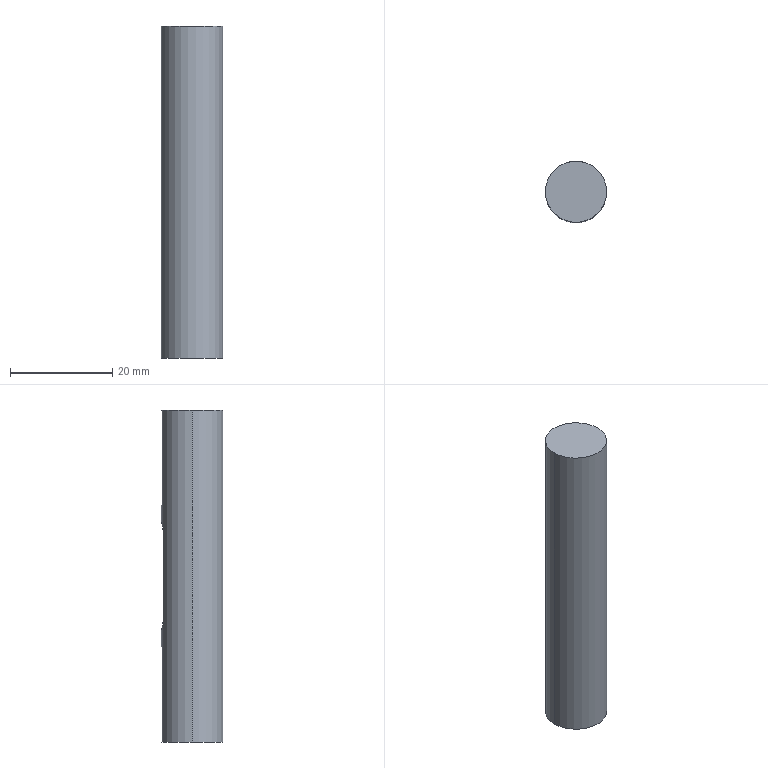Part | 1 solid | 10 faces | box 12 x 12 x 65 mm | volume 7199 mm3 | cylinder 5 | plane 5 | commonest cylinder face diameters 4 x3 12 x2
STEP:
#1=CARTESIAN_POINT('',(2.,5.657,24.));
#2=VERTEX_POINT('',#1);
#3=CARTESIAN_POINT('',(0.,6.,22.));
#4=VERTEX_POINT('',#3);
#5=CARTESIAN_POINT('',(2.,5.657,24.));
#6=CARTESIAN_POINT('',(2.,5.657,23.867));
#7=CARTESIAN_POINT('',(1.987,5.662,23.736));
#8=CARTESIAN_POINT('',(1.935,5.679,23.479));
#9=CARTESIAN_POINT('',(1.896,5.693,23.351));
#10=CARTESIAN_POINT('',(1.796,5.725,23.11));
#11=CARTESIAN_POINT('',(1.734,5.744,22.995));
#12=CARTESIAN_POINT('',(1.589,5.786,22.779));
#13=CARTESIAN_POINT('',(1.505,5.809,22.677));
#14=CARTESIAN_POINT('',(1.23,5.876,22.402));
#15=CARTESIAN_POINT('',(1.009,5.92,22.253));
#16=CARTESIAN_POINT('',(0.648,5.966,22.103));
#17=CARTESIAN_POINT('',(0.5209,5.979,22.065));
#18=CARTESIAN_POINT('',(0.2621,5.996,22.013));
#19=CARTESIAN_POINT('',(0.1316,6.,22.));
#20=CARTESIAN_POINT('',(0.,6.,22.));
#21=B_SPLINE_CURVE_WITH_KNOTS('',3,(#5,#6,#7,#8,#9,#10,#11,#12,#13,#14,#15,#16,#17,#18,#19,#20),.UNSPECIFIED.,.F.,.F.,(4,2,2,2,2,2,2,4),(0.,0.0003937,0.0007875,0.001181,0.001575,0.002362,0.002756,0.00315),.UNSPECIFIED.);
#22=EDGE_CURVE('',#2,#4,#21,.T.);
#23=ORIENTED_EDGE('',*,*,#22,.T.);
#24=CARTESIAN_POINT('',(0.,4.,22.));
#25=VERTEX_POINT('',#24);
#26=CARTESIAN_POINT('',(0.,10.,22.));
#27=DIRECTION('',(0.,-1.,0.));
#28=VECTOR('',#27,1000.);
#29=LINE('',#26,#28);
#30=EDGE_CURVE('',#4,#25,#29,.T.);
#31=ORIENTED_EDGE('',*,*,#30,.T.);
#32=CARTESIAN_POINT('',(2.,4.,24.));
#33=VERTEX_POINT('',#32);
#34=CARTESIAN_POINT('',(0.,4.,24.));
#35=DIRECTION('',(0.,1.,0.));
#36=DIRECTION('',(0.,0.,1.));
#37=AXIS2_PLACEMENT_3D('',#34,#35,#36);
#38=CIRCLE('',#37,2.);
#39=EDGE_CURVE('',#33,#25,#38,.T.);
#40=ORIENTED_EDGE('',*,*,#39,.F.);
#41=CARTESIAN_POINT('',(2.,10.,24.));
#42=DIRECTION('',(0.,-1.,0.));
#43=VECTOR('',#42,1000.);
#44=LINE('',#41,#43);
#45=EDGE_CURVE('',#2,#33,#44,.T.);
#46=ORIENTED_EDGE('',*,*,#45,.F.);
#47=EDGE_LOOP('',(#23,#31,#40,#46));
#48=FACE_OUTER_BOUND('',#47,.T.);
#49=CARTESIAN_POINT('',(0.,10.,24.));
#50=DIRECTION('',(0.,-1.,0.));
#51=DIRECTION('',(0.,0.,-1.));
#52=AXIS2_PLACEMENT_3D('',#49,#50,#51);
#53=CYLINDRICAL_SURFACE('',#52,2.);
#54=ADVANCED_FACE('',(#48),#53,.F.);
#55=ORIENTED_EDGE('',*,*,#22,.F.);
#56=CARTESIAN_POINT('',(2.,5.657,41.));
#57=VERTEX_POINT('',#56);
#58=CARTESIAN_POINT('',(2.,5.657,65.));
#59=DIRECTION('',(0.,0.,-1.));
#60=VECTOR('',#59,1000.);
#61=LINE('',#58,#60);
#62=EDGE_CURVE('',#57,#2,#61,.T.);
#63=ORIENTED_EDGE('',*,*,#62,.F.);
#64=CARTESIAN_POINT('',(-2.,5.657,41.));
#65=VERTEX_POINT('',#64);
#66=CARTESIAN_POINT('',(-2.,5.657,41.));
#67=CARTESIAN_POINT('',(-2.,5.657,41.133));
#68=CARTESIAN_POINT('',(-1.987,5.662,41.264));
#69=CARTESIAN_POINT('',(-1.935,5.679,41.521));
#70=CARTESIAN_POINT('',(-1.897,5.693,41.648));
#71=CARTESIAN_POINT('',(-1.796,5.725,41.89));
#72=CARTESIAN_POINT('',(-1.735,5.744,42.004));
#73=CARTESIAN_POINT('',(-1.59,5.786,42.221));
#74=CARTESIAN_POINT('',(-1.506,5.809,42.323));
#75=CARTESIAN_POINT('',(-1.231,5.875,42.597));
#76=CARTESIAN_POINT('',(-1.01,5.919,42.746));
#77=CARTESIAN_POINT('',(-0.6496,5.966,42.896));
#78=CARTESIAN_POINT('',(-0.5226,5.979,42.935));
#79=CARTESIAN_POINT('',(-0.264,5.996,42.987));
#80=CARTESIAN_POINT('',(-0.1336,6.,43.));
#81=CARTESIAN_POINT('',(0.1294,6.,43.));
#82=CARTESIAN_POINT('',(0.2629,5.996,42.987));
#83=CARTESIAN_POINT('',(0.5202,5.979,42.936));
#84=CARTESIAN_POINT('',(0.6454,5.966,42.898));
#85=CARTESIAN_POINT('',(0.8889,5.935,42.796));
#86=CARTESIAN_POINT('',(1.004,5.916,42.734));
#87=CARTESIAN_POINT('',(1.22,5.876,42.59));
#88=CARTESIAN_POINT('',(1.322,5.853,42.507));
#89=CARTESIAN_POINT('',(1.506,5.809,42.323));
#90=CARTESIAN_POINT('',(1.588,5.787,42.223));
#91=CARTESIAN_POINT('',(1.733,5.745,42.007));
#92=CARTESIAN_POINT('',(1.796,5.725,41.89));
#93=CARTESIAN_POINT('',(1.946,5.677,41.529));
#94=CARTESIAN_POINT('',(2.,5.657,41.266));
#95=CARTESIAN_POINT('',(2.,5.657,41.));
#96=B_SPLINE_CURVE_WITH_KNOTS('',3,(#66,#67,#68,#69,#70,#71,#72,#73,#74,#75,#76,#77,#78,#79,#80,#81,#82,#83,#84,#85,#86,#87,#88,#89,#90,#91,#92,#93,#94,#95),.UNSPECIFIED.,.F.,.F.,(4,2,2,2,2,2,2,2,2,2,2,2,2,2,4),(0.,0.0003935,0.000787,0.00118,0.001574,0.002361,0.002754,0.003148,0.003541,0.003935,0.004328,0.004722,0.005115,0.005509,0.006296),.UNSPECIFIED.);
#97=EDGE_CURVE('',#65,#57,#96,.T.);
#98=ORIENTED_EDGE('',*,*,#97,.F.);
#99=CARTESIAN_POINT('',(-2.,5.657,24.));
#100=VERTEX_POINT('',#99);
#101=CARTESIAN_POINT('',(-2.,5.657,65.));
#102=DIRECTION('',(0.,0.,1.));
#103=VECTOR('',#102,1000.);
#104=LINE('',#101,#103);
#105=EDGE_CURVE('',#100,#65,#104,.T.);
#106=ORIENTED_EDGE('',*,*,#105,.F.);
#107=CARTESIAN_POINT('',(0.,6.,22.));
#108=CARTESIAN_POINT('',(-0.1314,6.,22.));
#109=CARTESIAN_POINT('',(-0.2649,5.996,22.013));
#110=CARTESIAN_POINT('',(-0.5219,5.979,22.065));
#111=CARTESIAN_POINT('',(-0.647,5.966,22.103));
#112=CARTESIAN_POINT('',(-0.8902,5.935,22.204));
#113=CARTESIAN_POINT('',(-1.006,5.916,22.266));
#114=CARTESIAN_POINT('',(-1.221,5.875,22.411));
#115=CARTESIAN_POINT('',(-1.323,5.853,22.494));
#116=CARTESIAN_POINT('',(-1.507,5.809,22.678));
#117=CARTESIAN_POINT('',(-1.589,5.786,22.778));
#118=CARTESIAN_POINT('',(-1.733,5.745,22.994));
#119=CARTESIAN_POINT('',(-1.796,5.725,23.111));
#120=CARTESIAN_POINT('',(-1.946,5.677,23.471));
#121=CARTESIAN_POINT('',(-2.,5.657,23.734));
#122=CARTESIAN_POINT('',(-2.,5.657,24.));
#123=B_SPLINE_CURVE_WITH_KNOTS('',3,(#107,#108,#109,#110,#111,#112,#113,#114,#115,#116,#117,#118,#119,#120,#121,#122),.UNSPECIFIED.,.F.,.F.,(4,2,2,2,2,2,2,4),(0.00315,0.003543,0.003936,0.00433,0.004723,0.005116,0.005509,0.006296),.UNSPECIFIED.);
#124=EDGE_CURVE('',#4,#100,#123,.T.);
#125=ORIENTED_EDGE('',*,*,#124,.F.);
#126=EDGE_LOOP('',(#55,#63,#98,#106,#125));
#127=FACE_BOUND('',#126,.T.);
#128=CARTESIAN_POINT('',(6.,0.,65.));
#129=VERTEX_POINT('',#128);
#130=CARTESIAN_POINT('',(-6.,0.,65.));
#131=VERTEX_POINT('',#130);
#132=CARTESIAN_POINT('',(0.,0.,65.));
#133=DIRECTION('',(0.,0.,1.));
#134=DIRECTION('',(1.,0.,0.));
#135=AXIS2_PLACEMENT_3D('',#132,#133,#134);
#136=CIRCLE('',#135,6.);
#137=EDGE_CURVE('',#129,#131,#136,.T.);
#138=ORIENTED_EDGE('',*,*,#137,.F.);
#139=CARTESIAN_POINT('',(6.,0.,0.));
#140=VERTEX_POINT('',#139);
#141=CARTESIAN_POINT('',(6.,0.,65.));
#142=DIRECTION('',(0.,0.,-1.));
#143=VECTOR('',#142,1000.);
#144=LINE('',#141,#143);
#145=EDGE_CURVE('',#129,#140,#144,.T.);
#146=ORIENTED_EDGE('',*,*,#145,.T.);
#147=CARTESIAN_POINT('',(-6.,0.,0.));
#148=VERTEX_POINT('',#147);
#149=CARTESIAN_POINT('',(0.,0.,0.));
#150=DIRECTION('',(0.,0.,1.));
#151=DIRECTION('',(1.,0.,0.));
#152=AXIS2_PLACEMENT_3D('',#149,#150,#151);
#153=CIRCLE('',#152,6.);
#154=EDGE_CURVE('',#140,#148,#153,.T.);
#155=ORIENTED_EDGE('',*,*,#154,.T.);
#156=CARTESIAN_POINT('',(-6.,0.,65.));
#157=DIRECTION('',(0.,0.,-1.));
#158=VECTOR('',#157,1000.);
#159=LINE('',#156,#158);
#160=EDGE_CURVE('',#131,#148,#159,.T.);
#161=ORIENTED_EDGE('',*,*,#160,.F.);
#162=EDGE_LOOP('',(#138,#146,#155,#161));
#163=FACE_OUTER_BOUND('',#162,.T.);
#164=CARTESIAN_POINT('',(0.,0.,65.));
#165=DIRECTION('',(0.,0.,-1.));
#166=DIRECTION('',(-1.,0.,0.));
#167=AXIS2_PLACEMENT_3D('',#164,#165,#166);
#168=CYLINDRICAL_SURFACE('',#167,6.);
#169=ADVANCED_FACE('',(#127,#163),#168,.T.);
#170=ORIENTED_EDGE('',*,*,#145,.F.);
#171=CARTESIAN_POINT('',(0.,0.,65.));
#172=DIRECTION('',(0.,0.,1.));
#173=DIRECTION('',(1.,0.,0.));
#174=AXIS2_PLACEMENT_3D('',#171,#172,#173);
#175=CIRCLE('',#174,6.);
#176=EDGE_CURVE('',#131,#129,#175,.T.);
#177=ORIENTED_EDGE('',*,*,#176,.F.);
#178=ORIENTED_EDGE('',*,*,#160,.T.);
#179=CARTESIAN_POINT('',(0.,0.,0.));
#180=DIRECTION('',(0.,0.,1.));
#181=DIRECTION('',(1.,0.,0.));
#182=AXIS2_PLACEMENT_3D('',#179,#180,#181);
#183=CIRCLE('',#182,6.);
#184=EDGE_CURVE('',#148,#140,#183,.T.);
#185=ORIENTED_EDGE('',*,*,#184,.T.);
#186=EDGE_LOOP('',(#170,#177,#178,#185));
#187=FACE_OUTER_BOUND('',#186,.T.);
#188=CARTESIAN_POINT('',(0.,0.,65.));
#189=DIRECTION('',(0.,0.,-1.));
#190=DIRECTION('',(-1.,0.,0.));
#191=AXIS2_PLACEMENT_3D('',#188,#189,#190);
#192=CYLINDRICAL_SURFACE('',#191,6.);
#193=ADVANCED_FACE('',(#187),#192,.T.);
#194=ORIENTED_EDGE('',*,*,#176,.T.);
#195=ORIENTED_EDGE('',*,*,#137,.T.);
#196=EDGE_LOOP('',(#194,#195));
#197=FACE_OUTER_BOUND('',#196,.T.);
#198=CARTESIAN_POINT('',(0.,0.,65.));
#199=DIRECTION('',(0.,0.,1.));
#200=DIRECTION('',(1.,0.,0.));
#201=AXIS2_PLACEMENT_3D('',#198,#199,#200);
#202=PLANE('',#201);
#203=ADVANCED_FACE('',(#197),#202,.T.);
#204=ORIENTED_EDGE('',*,*,#184,.F.);
#205=ORIENTED_EDGE('',*,*,#154,.F.);
#206=EDGE_LOOP('',(#204,#205));
#207=FACE_OUTER_BOUND('',#206,.T.);
#208=CARTESIAN_POINT('',(0.,0.,0.));
#209=DIRECTION('',(0.,0.,1.));
#210=DIRECTION('',(1.,0.,0.));
#211=AXIS2_PLACEMENT_3D('',#208,#209,#210);
#212=PLANE('',#211);
#213=ADVANCED_FACE('',(#207),#212,.F.);
#214=ORIENTED_EDGE('',*,*,#30,.F.);
#215=ORIENTED_EDGE('',*,*,#124,.T.);
#216=CARTESIAN_POINT('',(-2.,4.,24.));
#217=VERTEX_POINT('',#216);
#218=CARTESIAN_POINT('',(-2.,10.,24.));
#219=DIRECTION('',(0.,-1.,0.));
#220=VECTOR('',#219,1000.);
#221=LINE('',#218,#220);
#222=EDGE_CURVE('',#100,#217,#221,.T.);
#223=ORIENTED_EDGE('',*,*,#222,.T.);
#224=CARTESIAN_POINT('',(0.,4.,24.));
#225=DIRECTION('',(0.,1.,0.));
#226=DIRECTION('',(0.,0.,1.));
#227=AXIS2_PLACEMENT_3D('',#224,#225,#226);
#228=CIRCLE('',#227,2.);
#229=EDGE_CURVE('',#25,#217,#228,.T.);
#230=ORIENTED_EDGE('',*,*,#229,.F.);
#231=EDGE_LOOP('',(#214,#215,#223,#230));
#232=FACE_OUTER_BOUND('',#231,.T.);
#233=CARTESIAN_POINT('',(0.,10.,24.));
#234=DIRECTION('',(0.,-1.,0.));
#235=DIRECTION('',(0.,0.,-1.));
#236=AXIS2_PLACEMENT_3D('',#233,#234,#235);
#237=CYLINDRICAL_SURFACE('',#236,2.);
#238=ADVANCED_FACE('',(#232),#237,.F.);
#239=ORIENTED_EDGE('',*,*,#105,.T.);
#240=CARTESIAN_POINT('',(-2.,4.,41.));
#241=VERTEX_POINT('',#240);
#242=CARTESIAN_POINT('',(-2.,10.,41.));
#243=DIRECTION('',(0.,-1.,0.));
#244=VECTOR('',#243,1000.);
#245=LINE('',#242,#244);
#246=EDGE_CURVE('',#65,#241,#245,.T.);
#247=ORIENTED_EDGE('',*,*,#246,.T.);
#248=CARTESIAN_POINT('',(-2.,4.,24.));
#249=DIRECTION('',(0.,0.,1.));
#250=VECTOR('',#249,1000.);
#251=LINE('',#248,#250);
#252=EDGE_CURVE('',#217,#241,#251,.T.);
#253=ORIENTED_EDGE('',*,*,#252,.F.);
#254=ORIENTED_EDGE('',*,*,#222,.F.);
#255=EDGE_LOOP('',(#239,#247,#253,#254));
#256=FACE_OUTER_BOUND('',#255,.T.);
#257=CARTESIAN_POINT('',(-2.,10.,24.));
#258=DIRECTION('',(1.,0.,0.));
#259=DIRECTION('',(0.,0.,-1.));
#260=AXIS2_PLACEMENT_3D('',#257,#258,#259);
#261=PLANE('',#260);
#262=ADVANCED_FACE('',(#256),#261,.T.);
#263=ORIENTED_EDGE('',*,*,#97,.T.);
#264=CARTESIAN_POINT('',(2.,4.,41.));
#265=VERTEX_POINT('',#264);
#266=CARTESIAN_POINT('',(2.,10.,41.));
#267=DIRECTION('',(0.,-1.,0.));
#268=VECTOR('',#267,1000.);
#269=LINE('',#266,#268);
#270=EDGE_CURVE('',#57,#265,#269,.T.);
#271=ORIENTED_EDGE('',*,*,#270,.T.);
#272=CARTESIAN_POINT('',(0.,4.,41.));
#273=DIRECTION('',(0.,1.,0.));
#274=DIRECTION('',(0.,0.,1.));
#275=AXIS2_PLACEMENT_3D('',#272,#273,#274);
#276=CIRCLE('',#275,2.);
#277=EDGE_CURVE('',#241,#265,#276,.T.);
#278=ORIENTED_EDGE('',*,*,#277,.F.);
#279=ORIENTED_EDGE('',*,*,#246,.F.);
#280=EDGE_LOOP('',(#263,#271,#278,#279));
#281=FACE_OUTER_BOUND('',#280,.T.);
#282=CARTESIAN_POINT('',(0.,10.,41.));
#283=DIRECTION('',(0.,-1.,0.));
#284=DIRECTION('',(0.,0.,-1.));
#285=AXIS2_PLACEMENT_3D('',#282,#283,#284);
#286=CYLINDRICAL_SURFACE('',#285,2.);
#287=ADVANCED_FACE('',(#281),#286,.F.);
#288=ORIENTED_EDGE('',*,*,#62,.T.);
#289=ORIENTED_EDGE('',*,*,#45,.T.);
#290=CARTESIAN_POINT('',(2.,4.,24.));
#291=DIRECTION('',(0.,0.,-1.));
#292=VECTOR('',#291,1000.);
#293=LINE('',#290,#292);
#294=EDGE_CURVE('',#265,#33,#293,.T.);
#295=ORIENTED_EDGE('',*,*,#294,.F.);
#296=ORIENTED_EDGE('',*,*,#270,.F.);
#297=EDGE_LOOP('',(#288,#289,#295,#296));
#298=FACE_OUTER_BOUND('',#297,.T.);
#299=CARTESIAN_POINT('',(2.,10.,24.));
#300=DIRECTION('',(-1.,0.,0.));
#301=DIRECTION('',(0.,0.,1.));
#302=AXIS2_PLACEMENT_3D('',#299,#300,#301);
#303=PLANE('',#302);
#304=ADVANCED_FACE('',(#298),#303,.T.);
#305=ORIENTED_EDGE('',*,*,#39,.T.);
#306=ORIENTED_EDGE('',*,*,#229,.T.);
#307=ORIENTED_EDGE('',*,*,#252,.T.);
#308=ORIENTED_EDGE('',*,*,#277,.T.);
#309=ORIENTED_EDGE('',*,*,#294,.T.);
#310=EDGE_LOOP('',(#305,#306,#307,#308,#309));
#311=FACE_OUTER_BOUND('',#310,.T.);
#312=CARTESIAN_POINT('',(0.,4.,24.));
#313=DIRECTION('',(0.,1.,0.));
#314=DIRECTION('',(0.,0.,1.));
#315=AXIS2_PLACEMENT_3D('',#312,#313,#314);
#316=PLANE('',#315);
#317=ADVANCED_FACE('',(#311),#316,.T.);
#318=CLOSED_SHELL('',(#54,#169,#193,#203,#213,#238,#262,#287,#304,#317));
#319=MANIFOLD_SOLID_BREP('',#318);
#320=CARTESIAN_POINT('',(0.,0.,0.));
#321=DIRECTION('',(0.,0.,1.));
#322=DIRECTION('',(1.,0.,0.));
#323=AXIS2_PLACEMENT_3D('',#320,#321,#322);
#324=(LENGTH_UNIT()NAMED_UNIT(*)SI_UNIT(.MILLI.,.METRE.));
#325=UNCERTAINTY_MEASURE_WITH_UNIT(LENGTH_MEASURE(0.00001),#324,'','');
#326=(NAMED_UNIT(*)PLANE_ANGLE_UNIT()SI_UNIT($,.RADIAN.));
#327=(NAMED_UNIT(*)SI_UNIT($,.STERADIAN.)SOLID_ANGLE_UNIT());
#328=(GEOMETRIC_REPRESENTATION_CONTEXT(3)GLOBAL_UNCERTAINTY_ASSIGNED_CONTEXT((#325))GLOBAL_UNIT_ASSIGNED_CONTEXT((#324,#326,#327))REPRESENTATION_CONTEXT('',''));
#329=ADVANCED_BREP_SHAPE_REPRESENTATION('',(#319,#323),#328);